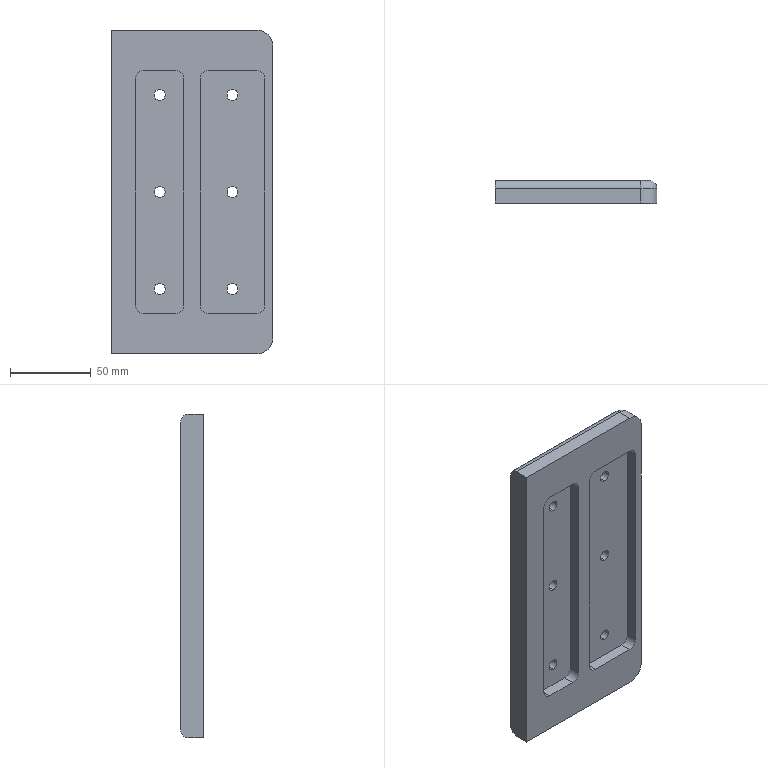Part | SolidWorks | features ICE 8, Fillet 3, HoleWzd 2, Chamfer 1, Extrusion 1, LPattern 1 | 1 solid | 43 faces | box 100 x 14 x 200 mm | volume 202593 mm3 | cylinder 25 | plane 16 | torus 2 | commonest cylinder face diameters 6.8 x12 10 x11 20 x2
STEP:
#1=CARTESIAN_POINT('',(-20.,14.,-63.4));
#2=VERTEX_POINT('',#1);
#3=CARTESIAN_POINT('',(-20.,14.,-56.6));
#4=VERTEX_POINT('',#3);
#5=CARTESIAN_POINT('',(-20.,14.,-60.));
#6=DIRECTION('',(0.,1.,0.));
#7=DIRECTION('',(0.,0.,1.));
#8=AXIS2_PLACEMENT_3D('',#5,#6,#7);
#9=CIRCLE('',#8,3.4);
#10=EDGE_CURVE('',#2,#4,#9,.T.);
#11=ORIENTED_EDGE('',*,*,#10,.T.);
#12=CARTESIAN_POINT('',(-20.,7.,-56.6));
#13=VERTEX_POINT('',#12);
#14=CARTESIAN_POINT('',(-20.,7.,-56.6));
#15=DIRECTION('',(0.,-1.,0.));
#16=VECTOR('',#15,1000.);
#17=LINE('',#14,#16);
#18=EDGE_CURVE('',#4,#13,#17,.T.);
#19=ORIENTED_EDGE('',*,*,#18,.T.);
#20=CARTESIAN_POINT('',(-20.,7.,-63.4));
#21=VERTEX_POINT('',#20);
#22=CARTESIAN_POINT('',(-20.,7.,-60.));
#23=DIRECTION('',(0.,-1.,0.));
#24=DIRECTION('',(0.,0.,-1.));
#25=AXIS2_PLACEMENT_3D('',#22,#23,#24);
#26=CIRCLE('',#25,3.4);
#27=EDGE_CURVE('',#13,#21,#26,.T.);
#28=ORIENTED_EDGE('',*,*,#27,.T.);
#29=CARTESIAN_POINT('',(-20.,7.,-63.4));
#30=DIRECTION('',(0.,-1.,0.));
#31=VECTOR('',#30,1000.);
#32=LINE('',#29,#31);
#33=EDGE_CURVE('',#2,#21,#32,.T.);
#34=ORIENTED_EDGE('',*,*,#33,.F.);
#35=EDGE_LOOP('',(#11,#19,#28,#34));
#36=FACE_OUTER_BOUND('',#35,.T.);
#37=CARTESIAN_POINT('',(-20.,7.,-60.));
#38=DIRECTION('',(0.,-1.,0.));
#39=DIRECTION('',(0.,0.,-1.));
#40=AXIS2_PLACEMENT_3D('',#37,#38,#39);
#41=CYLINDRICAL_SURFACE('',#40,3.4);
#42=ADVANCED_FACE('',(#36),#41,.F.);
#43=CARTESIAN_POINT('',(-20.,14.,-3.4));
#44=VERTEX_POINT('',#43);
#45=CARTESIAN_POINT('',(-20.,14.,3.4));
#46=VERTEX_POINT('',#45);
#47=CARTESIAN_POINT('',(-20.,14.,0.));
#48=DIRECTION('',(0.,1.,0.));
#49=DIRECTION('',(0.,0.,1.));
#50=AXIS2_PLACEMENT_3D('',#47,#48,#49);
#51=CIRCLE('',#50,3.4);
#52=EDGE_CURVE('',#44,#46,#51,.T.);
#53=ORIENTED_EDGE('',*,*,#52,.T.);
#54=CARTESIAN_POINT('',(-20.,7.,3.4));
#55=VERTEX_POINT('',#54);
#56=CARTESIAN_POINT('',(-20.,7.,3.4));
#57=DIRECTION('',(0.,-1.,0.));
#58=VECTOR('',#57,1000.);
#59=LINE('',#56,#58);
#60=EDGE_CURVE('',#46,#55,#59,.T.);
#61=ORIENTED_EDGE('',*,*,#60,.T.);
#62=CARTESIAN_POINT('',(-20.,7.,-3.4));
#63=VERTEX_POINT('',#62);
#64=CARTESIAN_POINT('',(-20.,7.,0.));
#65=DIRECTION('',(0.,-1.,0.));
#66=DIRECTION('',(0.,0.,-1.));
#67=AXIS2_PLACEMENT_3D('',#64,#65,#66);
#68=CIRCLE('',#67,3.4);
#69=EDGE_CURVE('',#55,#63,#68,.T.);
#70=ORIENTED_EDGE('',*,*,#69,.T.);
#71=CARTESIAN_POINT('',(-20.,7.,-3.4));
#72=DIRECTION('',(0.,-1.,0.));
#73=VECTOR('',#72,1000.);
#74=LINE('',#71,#73);
#75=EDGE_CURVE('',#44,#63,#74,.T.);
#76=ORIENTED_EDGE('',*,*,#75,.F.);
#77=EDGE_LOOP('',(#53,#61,#70,#76));
#78=FACE_OUTER_BOUND('',#77,.T.);
#79=CARTESIAN_POINT('',(-20.,7.,0.));
#80=DIRECTION('',(0.,-1.,0.));
#81=DIRECTION('',(0.,0.,-1.));
#82=AXIS2_PLACEMENT_3D('',#79,#80,#81);
#83=CYLINDRICAL_SURFACE('',#82,3.4);
#84=ADVANCED_FACE('',(#78),#83,.F.);
#85=CARTESIAN_POINT('',(-20.,14.,56.6));
#86=VERTEX_POINT('',#85);
#87=CARTESIAN_POINT('',(-20.,14.,63.4));
#88=VERTEX_POINT('',#87);
#89=CARTESIAN_POINT('',(-20.,14.,60.));
#90=DIRECTION('',(0.,1.,0.));
#91=DIRECTION('',(0.,0.,1.));
#92=AXIS2_PLACEMENT_3D('',#89,#90,#91);
#93=CIRCLE('',#92,3.4);
#94=EDGE_CURVE('',#86,#88,#93,.T.);
#95=ORIENTED_EDGE('',*,*,#94,.T.);
#96=CARTESIAN_POINT('',(-20.,7.,63.4));
#97=VERTEX_POINT('',#96);
#98=CARTESIAN_POINT('',(-20.,7.,63.4));
#99=DIRECTION('',(0.,-1.,0.));
#100=VECTOR('',#99,1000.);
#101=LINE('',#98,#100);
#102=EDGE_CURVE('',#88,#97,#101,.T.);
#103=ORIENTED_EDGE('',*,*,#102,.T.);
#104=CARTESIAN_POINT('',(-20.,7.,56.6));
#105=VERTEX_POINT('',#104);
#106=CARTESIAN_POINT('',(-20.,7.,60.));
#107=DIRECTION('',(0.,-1.,0.));
#108=DIRECTION('',(0.,0.,-1.));
#109=AXIS2_PLACEMENT_3D('',#106,#107,#108);
#110=CIRCLE('',#109,3.4);
#111=EDGE_CURVE('',#97,#105,#110,.T.);
#112=ORIENTED_EDGE('',*,*,#111,.T.);
#113=CARTESIAN_POINT('',(-20.,7.,56.6));
#114=DIRECTION('',(0.,-1.,0.));
#115=VECTOR('',#114,1000.);
#116=LINE('',#113,#115);
#117=EDGE_CURVE('',#86,#105,#116,.T.);
#118=ORIENTED_EDGE('',*,*,#117,.F.);
#119=EDGE_LOOP('',(#95,#103,#112,#118));
#120=FACE_OUTER_BOUND('',#119,.T.);
#121=CARTESIAN_POINT('',(-20.,7.,60.));
#122=DIRECTION('',(0.,-1.,0.));
#123=DIRECTION('',(0.,0.,-1.));
#124=AXIS2_PLACEMENT_3D('',#121,#122,#123);
#125=CYLINDRICAL_SURFACE('',#124,3.4);
#126=ADVANCED_FACE('',(#120),#125,.F.);
#127=CARTESIAN_POINT('',(25.,14.,-63.4));
#128=VERTEX_POINT('',#127);
#129=CARTESIAN_POINT('',(25.,14.,-56.6));
#130=VERTEX_POINT('',#129);
#131=CARTESIAN_POINT('',(25.,14.,-60.));
#132=DIRECTION('',(0.,1.,0.));
#133=DIRECTION('',(0.,0.,1.));
#134=AXIS2_PLACEMENT_3D('',#131,#132,#133);
#135=CIRCLE('',#134,3.4);
#136=EDGE_CURVE('',#128,#130,#135,.T.);
#137=ORIENTED_EDGE('',*,*,#136,.T.);
#138=CARTESIAN_POINT('',(25.,7.,-56.6));
#139=VERTEX_POINT('',#138);
#140=CARTESIAN_POINT('',(25.,7.,-56.6));
#141=DIRECTION('',(0.,-1.,0.));
#142=VECTOR('',#141,1000.);
#143=LINE('',#140,#142);
#144=EDGE_CURVE('',#130,#139,#143,.T.);
#145=ORIENTED_EDGE('',*,*,#144,.T.);
#146=CARTESIAN_POINT('',(25.,7.,-63.4));
#147=VERTEX_POINT('',#146);
#148=CARTESIAN_POINT('',(25.,7.,-60.));
#149=DIRECTION('',(0.,-1.,0.));
#150=DIRECTION('',(0.,0.,-1.));
#151=AXIS2_PLACEMENT_3D('',#148,#149,#150);
#152=CIRCLE('',#151,3.4);
#153=EDGE_CURVE('',#139,#147,#152,.T.);
#154=ORIENTED_EDGE('',*,*,#153,.T.);
#155=CARTESIAN_POINT('',(25.,7.,-63.4));
#156=DIRECTION('',(0.,-1.,0.));
#157=VECTOR('',#156,1000.);
#158=LINE('',#155,#157);
#159=EDGE_CURVE('',#128,#147,#158,.T.);
#160=ORIENTED_EDGE('',*,*,#159,.F.);
#161=EDGE_LOOP('',(#137,#145,#154,#160));
#162=FACE_OUTER_BOUND('',#161,.T.);
#163=CARTESIAN_POINT('',(25.,7.,-60.));
#164=DIRECTION('',(0.,-1.,0.));
#165=DIRECTION('',(0.,0.,-1.));
#166=AXIS2_PLACEMENT_3D('',#163,#164,#165);
#167=CYLINDRICAL_SURFACE('',#166,3.4);
#168=ADVANCED_FACE('',(#162),#167,.F.);
#169=CARTESIAN_POINT('',(25.,14.,-3.4));
#170=VERTEX_POINT('',#169);
#171=CARTESIAN_POINT('',(25.,14.,3.4));
#172=VERTEX_POINT('',#171);
#173=CARTESIAN_POINT('',(25.,14.,0.));
#174=DIRECTION('',(0.,1.,0.));
#175=DIRECTION('',(0.,0.,1.));
#176=AXIS2_PLACEMENT_3D('',#173,#174,#175);
#177=CIRCLE('',#176,3.4);
#178=EDGE_CURVE('',#170,#172,#177,.T.);
#179=ORIENTED_EDGE('',*,*,#178,.T.);
#180=CARTESIAN_POINT('',(25.,7.,3.4));
#181=VERTEX_POINT('',#180);
#182=CARTESIAN_POINT('',(25.,7.,3.4));
#183=DIRECTION('',(0.,-1.,0.));
#184=VECTOR('',#183,1000.);
#185=LINE('',#182,#184);
#186=EDGE_CURVE('',#172,#181,#185,.T.);
#187=ORIENTED_EDGE('',*,*,#186,.T.);
#188=CARTESIAN_POINT('',(25.,7.,-3.4));
#189=VERTEX_POINT('',#188);
#190=CARTESIAN_POINT('',(25.,7.,0.));
#191=DIRECTION('',(0.,-1.,0.));
#192=DIRECTION('',(0.,0.,-1.));
#193=AXIS2_PLACEMENT_3D('',#190,#191,#192);
#194=CIRCLE('',#193,3.4);
#195=EDGE_CURVE('',#181,#189,#194,.T.);
#196=ORIENTED_EDGE('',*,*,#195,.T.);
#197=CARTESIAN_POINT('',(25.,7.,-3.4));
#198=DIRECTION('',(0.,-1.,0.));
#199=VECTOR('',#198,1000.);
#200=LINE('',#197,#199);
#201=EDGE_CURVE('',#170,#189,#200,.T.);
#202=ORIENTED_EDGE('',*,*,#201,.F.);
#203=EDGE_LOOP('',(#179,#187,#196,#202));
#204=FACE_OUTER_BOUND('',#203,.T.);
#205=CARTESIAN_POINT('',(25.,7.,0.));
#206=DIRECTION('',(0.,-1.,0.));
#207=DIRECTION('',(0.,0.,-1.));
#208=AXIS2_PLACEMENT_3D('',#205,#206,#207);
#209=CYLINDRICAL_SURFACE('',#208,3.4);
#210=ADVANCED_FACE('',(#204),#209,.F.);
#211=CARTESIAN_POINT('',(25.,14.,56.6));
#212=VERTEX_POINT('',#211);
#213=CARTESIAN_POINT('',(25.,14.,63.4));
#214=VERTEX_POINT('',#213);
#215=CARTESIAN_POINT('',(25.,14.,60.));
#216=DIRECTION('',(0.,1.,0.));
#217=DIRECTION('',(0.,0.,1.));
#218=AXIS2_PLACEMENT_3D('',#215,#216,#217);
#219=CIRCLE('',#218,3.4);
#220=EDGE_CURVE('',#212,#214,#219,.T.);
#221=ORIENTED_EDGE('',*,*,#220,.T.);
#222=CARTESIAN_POINT('',(25.,7.,63.4));
#223=VERTEX_POINT('',#222);
#224=CARTESIAN_POINT('',(25.,7.,63.4));
#225=DIRECTION('',(0.,-1.,0.));
#226=VECTOR('',#225,1000.);
#227=LINE('',#224,#226);
#228=EDGE_CURVE('',#214,#223,#227,.T.);
#229=ORIENTED_EDGE('',*,*,#228,.T.);
#230=CARTESIAN_POINT('',(25.,7.,56.6));
#231=VERTEX_POINT('',#230);
#232=CARTESIAN_POINT('',(25.,7.,60.));
#233=DIRECTION('',(0.,-1.,0.));
#234=DIRECTION('',(0.,0.,-1.));
#235=AXIS2_PLACEMENT_3D('',#232,#233,#234);
#236=CIRCLE('',#235,3.4);
#237=EDGE_CURVE('',#223,#231,#236,.T.);
#238=ORIENTED_EDGE('',*,*,#237,.T.);
#239=CARTESIAN_POINT('',(25.,7.,56.6));
#240=DIRECTION('',(0.,-1.,0.));
#241=VECTOR('',#240,1000.);
#242=LINE('',#239,#241);
#243=EDGE_CURVE('',#212,#231,#242,.T.);
#244=ORIENTED_EDGE('',*,*,#243,.F.);
#245=EDGE_LOOP('',(#221,#229,#238,#244));
#246=FACE_OUTER_BOUND('',#245,.T.);
#247=CARTESIAN_POINT('',(25.,7.,60.));
#248=DIRECTION('',(0.,-1.,0.));
#249=DIRECTION('',(0.,0.,-1.));
#250=AXIS2_PLACEMENT_3D('',#247,#248,#249);
#251=CYLINDRICAL_SURFACE('',#250,3.4);
#252=ADVANCED_FACE('',(#246),#251,.F.);
#253=CARTESIAN_POINT('',(-30.,0.,-75.));
#254=VERTEX_POINT('',#253);
#255=CARTESIAN_POINT('',(-10.,0.,-75.));
#256=VERTEX_POINT('',#255);
#257=CARTESIAN_POINT('',(-45.,0.,-75.));
#258=DIRECTION('',(1.,0.,0.));
#259=VECTOR('',#258,1000.);
#260=LINE('',#257,#259);
#261=EDGE_CURVE('',#254,#256,#260,.T.);
#262=ORIENTED_EDGE('',*,*,#261,.F.);
#263=CARTESIAN_POINT('',(-35.,0.,-70.));
#264=VERTEX_POINT('',#263);
#265=CARTESIAN_POINT('',(-30.,0.,-70.));
#266=DIRECTION('',(0.,1.,0.));
#267=DIRECTION('',(0.,0.,1.));
#268=AXIS2_PLACEMENT_3D('',#265,#266,#267);
#269=CIRCLE('',#268,5.);
#270=EDGE_CURVE('',#254,#264,#269,.T.);
#271=ORIENTED_EDGE('',*,*,#270,.T.);
#272=CARTESIAN_POINT('',(-35.,0.,70.));
#273=VERTEX_POINT('',#272);
#274=CARTESIAN_POINT('',(-35.,0.,75.));
#275=DIRECTION('',(0.,0.,1.));
#276=VECTOR('',#275,1000.);
#277=LINE('',#274,#276);
#278=EDGE_CURVE('',#264,#273,#277,.T.);
#279=ORIENTED_EDGE('',*,*,#278,.T.);
#280=CARTESIAN_POINT('',(-30.,0.,75.));
#281=VERTEX_POINT('',#280);
#282=CARTESIAN_POINT('',(-30.,0.,70.));
#283=DIRECTION('',(0.,1.,0.));
#284=DIRECTION('',(0.,0.,1.));
#285=AXIS2_PLACEMENT_3D('',#282,#283,#284);
#286=CIRCLE('',#285,5.);
#287=EDGE_CURVE('',#273,#281,#286,.T.);
#288=ORIENTED_EDGE('',*,*,#287,.T.);
#289=CARTESIAN_POINT('',(-10.,0.,75.));
#290=VERTEX_POINT('',#289);
#291=CARTESIAN_POINT('',(-45.,0.,75.));
#292=DIRECTION('',(-1.,0.,0.));
#293=VECTOR('',#292,1000.);
#294=LINE('',#291,#293);
#295=EDGE_CURVE('',#290,#281,#294,.T.);
#296=ORIENTED_EDGE('',*,*,#295,.F.);
#297=CARTESIAN_POINT('',(-5.,0.,70.));
#298=VERTEX_POINT('',#297);
#299=CARTESIAN_POINT('',(-10.,0.,70.));
#300=DIRECTION('',(0.,1.,0.));
#301=DIRECTION('',(0.,0.,1.));
#302=AXIS2_PLACEMENT_3D('',#299,#300,#301);
#303=CIRCLE('',#302,5.);
#304=EDGE_CURVE('',#290,#298,#303,.T.);
#305=ORIENTED_EDGE('',*,*,#304,.T.);
#306=CARTESIAN_POINT('',(-5.,0.,-70.));
#307=VERTEX_POINT('',#306);
#308=CARTESIAN_POINT('',(-5.,0.,75.));
#309=DIRECTION('',(0.,0.,1.));
#310=VECTOR('',#309,1000.);
#311=LINE('',#308,#310);
#312=EDGE_CURVE('',#307,#298,#311,.T.);
#313=ORIENTED_EDGE('',*,*,#312,.F.);
#314=CARTESIAN_POINT('',(-10.,0.,-70.));
#315=DIRECTION('',(0.,1.,0.));
#316=DIRECTION('',(0.,0.,1.));
#317=AXIS2_PLACEMENT_3D('',#314,#315,#316);
#318=CIRCLE('',#317,5.);
#319=EDGE_CURVE('',#307,#256,#318,.T.);
#320=ORIENTED_EDGE('',*,*,#319,.T.);
#321=EDGE_LOOP('',(#262,#271,#279,#288,#296,#305,#313,#320));
#322=FACE_BOUND('',#321,.T.);
#323=CARTESIAN_POINT('',(40.,0.,-100.));
#324=VERTEX_POINT('',#323);
#325=CARTESIAN_POINT('',(-50.,0.,-100.));
#326=VERTEX_POINT('',#325);
#327=CARTESIAN_POINT('',(-50.,0.,-100.));
#328=DIRECTION('',(-1.,0.,0.));
#329=VECTOR('',#328,1000.);
#330=LINE('',#327,#329);
#331=EDGE_CURVE('',#324,#326,#330,.T.);
#332=ORIENTED_EDGE('',*,*,#331,.F.);
#333=CARTESIAN_POINT('',(50.,0.,-90.));
#334=VERTEX_POINT('',#333);
#335=CARTESIAN_POINT('',(40.,0.,-90.));
#336=DIRECTION('',(0.,-1.,0.));
#337=DIRECTION('',(0.,0.,1.));
#338=AXIS2_PLACEMENT_3D('',#335,#336,#337);
#339=CIRCLE('',#338,10.);
#340=EDGE_CURVE('',#324,#334,#339,.T.);
#341=ORIENTED_EDGE('',*,*,#340,.T.);
#342=CARTESIAN_POINT('',(50.,0.,90.));
#343=VERTEX_POINT('',#342);
#344=CARTESIAN_POINT('',(50.,0.,-100.));
#345=DIRECTION('',(0.,0.,-1.));
#346=VECTOR('',#345,1000.);
#347=LINE('',#344,#346);
#348=EDGE_CURVE('',#343,#334,#347,.T.);
#349=ORIENTED_EDGE('',*,*,#348,.F.);
#350=CARTESIAN_POINT('',(40.,0.,100.));
#351=VERTEX_POINT('',#350);
#352=CARTESIAN_POINT('',(40.,0.,90.));
#353=DIRECTION('',(0.,-1.,0.));
#354=DIRECTION('',(0.,0.,1.));
#355=AXIS2_PLACEMENT_3D('',#352,#353,#354);
#356=CIRCLE('',#355,10.);
#357=EDGE_CURVE('',#343,#351,#356,.T.);
#358=ORIENTED_EDGE('',*,*,#357,.T.);
#359=CARTESIAN_POINT('',(-50.,0.,100.));
#360=VERTEX_POINT('',#359);
#361=CARTESIAN_POINT('',(-50.,0.,100.));
#362=DIRECTION('',(1.,0.,0.));
#363=VECTOR('',#362,1000.);
#364=LINE('',#361,#363);
#365=EDGE_CURVE('',#360,#351,#364,.T.);
#366=ORIENTED_EDGE('',*,*,#365,.F.);
#367=CARTESIAN_POINT('',(-50.,0.,-100.));
#368=DIRECTION('',(0.,0.,1.));
#369=VECTOR('',#368,1000.);
#370=LINE('',#367,#369);
#371=EDGE_CURVE('',#326,#360,#370,.T.);
#372=ORIENTED_EDGE('',*,*,#371,.F.);
#373=EDGE_LOOP('',(#332,#341,#349,#358,#366,#372));
#374=FACE_OUTER_BOUND('',#373,.T.);
#375=CARTESIAN_POINT('',(40.,0.,75.));
#376=VERTEX_POINT('',#375);
#377=CARTESIAN_POINT('',(10.,0.,75.));
#378=VERTEX_POINT('',#377);
#379=CARTESIAN_POINT('',(45.,0.,75.));
#380=DIRECTION('',(-1.,0.,0.));
#381=VECTOR('',#380,1000.);
#382=LINE('',#379,#381);
#383=EDGE_CURVE('',#376,#378,#382,.T.);
#384=ORIENTED_EDGE('',*,*,#383,.F.);
#385=CARTESIAN_POINT('',(45.,0.,70.));
#386=VERTEX_POINT('',#385);
#387=CARTESIAN_POINT('',(40.,0.,70.));
#388=DIRECTION('',(0.,1.,0.));
#389=DIRECTION('',(0.,0.,1.));
#390=AXIS2_PLACEMENT_3D('',#387,#388,#389);
#391=CIRCLE('',#390,5.);
#392=EDGE_CURVE('',#376,#386,#391,.T.);
#393=ORIENTED_EDGE('',*,*,#392,.T.);
#394=CARTESIAN_POINT('',(45.,0.,-70.));
#395=VERTEX_POINT('',#394);
#396=CARTESIAN_POINT('',(45.,0.,75.));
#397=DIRECTION('',(0.,0.,1.));
#398=VECTOR('',#397,1000.);
#399=LINE('',#396,#398);
#400=EDGE_CURVE('',#395,#386,#399,.T.);
#401=ORIENTED_EDGE('',*,*,#400,.F.);
#402=CARTESIAN_POINT('',(40.,0.,-75.));
#403=VERTEX_POINT('',#402);
#404=CARTESIAN_POINT('',(40.,0.,-70.));
#405=DIRECTION('',(0.,1.,0.));
#406=DIRECTION('',(0.,0.,1.));
#407=AXIS2_PLACEMENT_3D('',#404,#405,#406);
#408=CIRCLE('',#407,5.);
#409=EDGE_CURVE('',#395,#403,#408,.T.);
#410=ORIENTED_EDGE('',*,*,#409,.T.);
#411=CARTESIAN_POINT('',(10.,0.,-75.));
#412=VERTEX_POINT('',#411);
#413=CARTESIAN_POINT('',(45.,0.,-75.));
#414=DIRECTION('',(1.,0.,0.));
#415=VECTOR('',#414,1000.);
#416=LINE('',#413,#415);
#417=EDGE_CURVE('',#412,#403,#416,.T.);
#418=ORIENTED_EDGE('',*,*,#417,.F.);
#419=CARTESIAN_POINT('',(5.,0.,-70.));
#420=VERTEX_POINT('',#419);
#421=CARTESIAN_POINT('',(10.,0.,-70.));
#422=DIRECTION('',(0.,1.,0.));
#423=DIRECTION('',(0.,0.,1.));
#424=AXIS2_PLACEMENT_3D('',#421,#422,#423);
#425=CIRCLE('',#424,5.);
#426=EDGE_CURVE('',#412,#420,#425,.T.);
#427=ORIENTED_EDGE('',*,*,#426,.T.);
#428=CARTESIAN_POINT('',(5.,0.,70.));
#429=VERTEX_POINT('',#428);
#430=CARTESIAN_POINT('',(5.,0.,75.));
#431=DIRECTION('',(0.,0.,-1.));
#432=VECTOR('',#431,1000.);
#433=LINE('',#430,#432);
#434=EDGE_CURVE('',#429,#420,#433,.T.);
#435=ORIENTED_EDGE('',*,*,#434,.F.);
#436=CARTESIAN_POINT('',(10.,0.,70.));
#437=DIRECTION('',(0.,1.,0.));
#438=DIRECTION('',(0.,0.,1.));
#439=AXIS2_PLACEMENT_3D('',#436,#437,#438);
#440=CIRCLE('',#439,5.);
#441=EDGE_CURVE('',#429,#378,#440,.T.);
#442=ORIENTED_EDGE('',*,*,#441,.T.);
#443=EDGE_LOOP('',(#384,#393,#401,#410,#418,#427,#435,#442));
#444=FACE_BOUND('',#443,.T.);
#445=CARTESIAN_POINT('',(0.,0.,0.));
#446=DIRECTION('',(0.,1.,0.));
#447=DIRECTION('',(0.,0.,1.));
#448=AXIS2_PLACEMENT_3D('',#445,#446,#447);
#449=PLANE('',#448);
#450=ADVANCED_FACE('',(#322,#374,#444),#449,.F.);
#451=CARTESIAN_POINT('',(50.,9.,-90.));
#452=VERTEX_POINT('',#451);
#453=CARTESIAN_POINT('',(50.,14.,-90.));
#454=DIRECTION('',(0.,1.,0.));
#455=VECTOR('',#454,1000.);
#456=LINE('',#453,#455);
#457=EDGE_CURVE('',#334,#452,#456,.T.);
#458=ORIENTED_EDGE('',*,*,#457,.T.);
#459=CARTESIAN_POINT('',(50.,9.,90.));
#460=VERTEX_POINT('',#459);
#461=CARTESIAN_POINT('',(50.,9.,90.));
#462=DIRECTION('',(0.,0.,1.));
#463=VECTOR('',#462,1000.);
#464=LINE('',#461,#463);
#465=EDGE_CURVE('',#452,#460,#464,.T.);
#466=ORIENTED_EDGE('',*,*,#465,.T.);
#467=CARTESIAN_POINT('',(50.,14.,90.));
#468=DIRECTION('',(0.,-1.,0.));
#469=VECTOR('',#468,1000.);
#470=LINE('',#467,#469);
#471=EDGE_CURVE('',#460,#343,#470,.T.);
#472=ORIENTED_EDGE('',*,*,#471,.T.);
#473=ORIENTED_EDGE('',*,*,#348,.T.);
#474=EDGE_LOOP('',(#458,#466,#472,#473));
#475=FACE_OUTER_BOUND('',#474,.T.);
#476=CARTESIAN_POINT('',(50.,14.,-100.));
#477=DIRECTION('',(-1.,0.,0.));
#478=DIRECTION('',(0.,0.,1.));
#479=AXIS2_PLACEMENT_3D('',#476,#477,#478);
#480=PLANE('',#479);
#481=ADVANCED_FACE('',(#475),#480,.F.);
#482=CARTESIAN_POINT('',(-50.,9.,-100.));
#483=VERTEX_POINT('',#482);
#484=CARTESIAN_POINT('',(-50.,14.,-100.));
#485=DIRECTION('',(0.,-1.,0.));
#486=VECTOR('',#485,1000.);
#487=LINE('',#484,#486);
#488=EDGE_CURVE('',#483,#326,#487,.T.);
#489=ORIENTED_EDGE('',*,*,#488,.F.);
#490=CARTESIAN_POINT('',(40.,9.,-100.));
#491=VERTEX_POINT('',#490);
#492=CARTESIAN_POINT('',(40.,9.,-100.));
#493=DIRECTION('',(1.,0.,0.));
#494=VECTOR('',#493,1000.);
#495=LINE('',#492,#494);
#496=EDGE_CURVE('',#483,#491,#495,.T.);
#497=ORIENTED_EDGE('',*,*,#496,.T.);
#498=CARTESIAN_POINT('',(40.,14.,-100.));
#499=DIRECTION('',(0.,-1.,0.));
#500=VECTOR('',#499,1000.);
#501=LINE('',#498,#500);
#502=EDGE_CURVE('',#491,#324,#501,.T.);
#503=ORIENTED_EDGE('',*,*,#502,.T.);
#504=ORIENTED_EDGE('',*,*,#331,.T.);
#505=EDGE_LOOP('',(#489,#497,#503,#504));
#506=FACE_OUTER_BOUND('',#505,.T.);
#507=CARTESIAN_POINT('',(-50.,14.,-100.));
#508=DIRECTION('',(0.,0.,1.));
#509=DIRECTION('',(1.,0.,0.));
#510=AXIS2_PLACEMENT_3D('',#507,#508,#509);
#511=PLANE('',#510);
#512=ADVANCED_FACE('',(#506),#511,.F.);
#513=CARTESIAN_POINT('',(-50.,9.,100.));
#514=VERTEX_POINT('',#513);
#515=CARTESIAN_POINT('',(-50.,14.,100.));
#516=DIRECTION('',(0.,-1.,0.));
#517=VECTOR('',#516,1000.);
#518=LINE('',#515,#517);
#519=EDGE_CURVE('',#514,#360,#518,.T.);
#520=ORIENTED_EDGE('',*,*,#519,.F.);
#521=CARTESIAN_POINT('',(-50.,14.,95.));
#522=VERTEX_POINT('',#521);
#523=CARTESIAN_POINT('',(-50.,9.,95.));
#524=DIRECTION('',(-1.,0.,0.));
#525=DIRECTION('',(0.,0.,-1.));
#526=AXIS2_PLACEMENT_3D('',#523,#524,#525);
#527=CIRCLE('',#526,5.);
#528=EDGE_CURVE('',#514,#522,#527,.T.);
#529=ORIENTED_EDGE('',*,*,#528,.T.);
#530=CARTESIAN_POINT('',(-50.,14.,-95.));
#531=VERTEX_POINT('',#530);
#532=CARTESIAN_POINT('',(-50.,14.,-100.));
#533=DIRECTION('',(0.,0.,1.));
#534=VECTOR('',#533,1000.);
#535=LINE('',#532,#534);
#536=EDGE_CURVE('',#531,#522,#535,.T.);
#537=ORIENTED_EDGE('',*,*,#536,.F.);
#538=CARTESIAN_POINT('',(-50.,9.,-95.));
#539=DIRECTION('',(-1.,0.,0.));
#540=DIRECTION('',(0.,0.,-1.));
#541=AXIS2_PLACEMENT_3D('',#538,#539,#540);
#542=CIRCLE('',#541,5.);
#543=EDGE_CURVE('',#531,#483,#542,.T.);
#544=ORIENTED_EDGE('',*,*,#543,.T.);
#545=ORIENTED_EDGE('',*,*,#488,.T.);
#546=ORIENTED_EDGE('',*,*,#371,.T.);
#547=EDGE_LOOP('',(#520,#529,#537,#544,#545,#546));
#548=FACE_OUTER_BOUND('',#547,.T.);
#549=CARTESIAN_POINT('',(-50.,14.,-100.));
#550=DIRECTION('',(1.,0.,0.));
#551=DIRECTION('',(0.,0.,-1.));
#552=AXIS2_PLACEMENT_3D('',#549,#550,#551);
#553=PLANE('',#552);
#554=ADVANCED_FACE('',(#548),#553,.F.);
#555=CARTESIAN_POINT('',(40.,9.,100.));
#556=VERTEX_POINT('',#555);
#557=CARTESIAN_POINT('',(40.,14.,100.));
#558=DIRECTION('',(0.,1.,0.));
#559=VECTOR('',#558,1000.);
#560=LINE('',#557,#559);
#561=EDGE_CURVE('',#351,#556,#560,.T.);
#562=ORIENTED_EDGE('',*,*,#561,.T.);
#563=CARTESIAN_POINT('',(-50.,9.,100.));
#564=DIRECTION('',(-1.,0.,0.));
#565=VECTOR('',#564,1000.);
#566=LINE('',#563,#565);
#567=EDGE_CURVE('',#556,#514,#566,.T.);
#568=ORIENTED_EDGE('',*,*,#567,.T.);
#569=ORIENTED_EDGE('',*,*,#519,.T.);
#570=ORIENTED_EDGE('',*,*,#365,.T.);
#571=EDGE_LOOP('',(#562,#568,#569,#570));
#572=FACE_OUTER_BOUND('',#571,.T.);
#573=CARTESIAN_POINT('',(-50.,14.,100.));
#574=DIRECTION('',(0.,0.,-1.));
#575=DIRECTION('',(-1.,0.,0.));
#576=AXIS2_PLACEMENT_3D('',#573,#574,#575);
#577=PLANE('',#576);
#578=ADVANCED_FACE('',(#572),#577,.F.);
#579=ORIENTED_EDGE('',*,*,#10,.F.);
#580=CARTESIAN_POINT('',(-20.,14.,-60.));
#581=DIRECTION('',(0.,1.,0.));
#582=DIRECTION('',(0.,0.,1.));
#583=AXIS2_PLACEMENT_3D('',#580,#581,#582);
#584=CIRCLE('',#583,3.4);
#585=EDGE_CURVE('',#4,#2,#584,.T.);
#586=ORIENTED_EDGE('',*,*,#585,.F.);
#587=EDGE_LOOP('',(#579,#586));
#588=FACE_BOUND('',#587,.T.);
#589=ORIENTED_EDGE('',*,*,#52,.F.);
#590=CARTESIAN_POINT('',(-20.,14.,0.));
#591=DIRECTION('',(0.,1.,0.));
#592=DIRECTION('',(0.,0.,1.));
#593=AXIS2_PLACEMENT_3D('',#590,#591,#592);
#594=CIRCLE('',#593,3.4);
#595=EDGE_CURVE('',#46,#44,#594,.T.);
#596=ORIENTED_EDGE('',*,*,#595,.F.);
#597=EDGE_LOOP('',(#589,#596));
#598=FACE_BOUND('',#597,.T.);
#599=ORIENTED_EDGE('',*,*,#94,.F.);
#600=CARTESIAN_POINT('',(-20.,14.,60.));
#601=DIRECTION('',(0.,1.,0.));
#602=DIRECTION('',(0.,0.,1.));
#603=AXIS2_PLACEMENT_3D('',#600,#601,#602);
#604=CIRCLE('',#603,3.4);
#605=EDGE_CURVE('',#88,#86,#604,.T.);
#606=ORIENTED_EDGE('',*,*,#605,.F.);
#607=EDGE_LOOP('',(#599,#606));
#608=FACE_BOUND('',#607,.T.);
#609=ORIENTED_EDGE('',*,*,#136,.F.);
#610=CARTESIAN_POINT('',(25.,14.,-60.));
#611=DIRECTION('',(0.,1.,0.));
#612=DIRECTION('',(0.,0.,1.));
#613=AXIS2_PLACEMENT_3D('',#610,#611,#612);
#614=CIRCLE('',#613,3.4);
#615=EDGE_CURVE('',#130,#128,#614,.T.);
#616=ORIENTED_EDGE('',*,*,#615,.F.);
#617=EDGE_LOOP('',(#609,#616));
#618=FACE_BOUND('',#617,.T.);
#619=ORIENTED_EDGE('',*,*,#178,.F.);
#620=CARTESIAN_POINT('',(25.,14.,0.));
#621=DIRECTION('',(0.,1.,0.));
#622=DIRECTION('',(0.,0.,1.));
#623=AXIS2_PLACEMENT_3D('',#620,#621,#622);
#624=CIRCLE('',#623,3.4);
#625=EDGE_CURVE('',#172,#170,#624,.T.);
#626=ORIENTED_EDGE('',*,*,#625,.F.);
#627=EDGE_LOOP('',(#619,#626));
#628=FACE_BOUND('',#627,.T.);
#629=ORIENTED_EDGE('',*,*,#220,.F.);
#630=CARTESIAN_POINT('',(25.,14.,60.));
#631=DIRECTION('',(0.,1.,0.));
#632=DIRECTION('',(0.,0.,1.));
#633=AXIS2_PLACEMENT_3D('',#630,#631,#632);
#634=CIRCLE('',#633,3.4);
#635=EDGE_CURVE('',#214,#212,#634,.T.);
#636=ORIENTED_EDGE('',*,*,#635,.F.);
#637=EDGE_LOOP('',(#629,#636));
#638=FACE_BOUND('',#637,.T.);
#639=ORIENTED_EDGE('',*,*,#536,.T.);
#640=CARTESIAN_POINT('',(40.,14.,95.));
#641=VERTEX_POINT('',#640);
#642=CARTESIAN_POINT('',(40.,14.,95.));
#643=DIRECTION('',(1.,0.,0.));
#644=VECTOR('',#643,1000.);
#645=LINE('',#642,#644);
#646=EDGE_CURVE('',#522,#641,#645,.T.);
#647=ORIENTED_EDGE('',*,*,#646,.T.);
#648=CARTESIAN_POINT('',(45.,14.,90.));
#649=VERTEX_POINT('',#648);
#650=CARTESIAN_POINT('',(40.,14.,90.));
#651=DIRECTION('',(0.,1.,0.));
#652=DIRECTION('',(0.,0.,1.));
#653=AXIS2_PLACEMENT_3D('',#650,#651,#652);
#654=CIRCLE('',#653,5.);
#655=EDGE_CURVE('',#641,#649,#654,.T.);
#656=ORIENTED_EDGE('',*,*,#655,.T.);
#657=CARTESIAN_POINT('',(45.,14.,-90.));
#658=VERTEX_POINT('',#657);
#659=CARTESIAN_POINT('',(45.,14.,-90.));
#660=DIRECTION('',(0.,0.,-1.));
#661=VECTOR('',#660,1000.);
#662=LINE('',#659,#661);
#663=EDGE_CURVE('',#649,#658,#662,.T.);
#664=ORIENTED_EDGE('',*,*,#663,.T.);
#665=CARTESIAN_POINT('',(40.,14.,-95.));
#666=VERTEX_POINT('',#665);
#667=CARTESIAN_POINT('',(40.,14.,-90.));
#668=DIRECTION('',(0.,1.,0.));
#669=DIRECTION('',(0.,0.,1.));
#670=AXIS2_PLACEMENT_3D('',#667,#668,#669);
#671=CIRCLE('',#670,5.);
#672=EDGE_CURVE('',#658,#666,#671,.T.);
#673=ORIENTED_EDGE('',*,*,#672,.T.);
#674=CARTESIAN_POINT('',(-50.,14.,-95.));
#675=DIRECTION('',(-1.,0.,0.));
#676=VECTOR('',#675,1000.);
#677=LINE('',#674,#676);
#678=EDGE_CURVE('',#666,#531,#677,.T.);
#679=ORIENTED_EDGE('',*,*,#678,.T.);
#680=EDGE_LOOP('',(#639,#647,#656,#664,#673,#679));
#681=FACE_OUTER_BOUND('',#680,.T.);
#682=CARTESIAN_POINT('',(0.,14.,0.));
#683=DIRECTION('',(0.,1.,0.));
#684=DIRECTION('',(0.,0.,1.));
#685=AXIS2_PLACEMENT_3D('',#682,#683,#684);
#686=PLANE('',#685);
#687=ADVANCED_FACE('',(#588,#598,#608,#618,#628,#638,#681),#686,.T.);
#688=ORIENTED_EDGE('',*,*,#502,.F.);
#689=CARTESIAN_POINT('',(40.,9.,-90.));
#690=DIRECTION('',(0.,-1.,0.));
#691=DIRECTION('',(0.,0.,1.));
#692=AXIS2_PLACEMENT_3D('',#689,#690,#691);
#693=CIRCLE('',#692,10.);
#694=EDGE_CURVE('',#491,#452,#693,.T.);
#695=ORIENTED_EDGE('',*,*,#694,.T.);
#696=ORIENTED_EDGE('',*,*,#457,.F.);
#697=ORIENTED_EDGE('',*,*,#340,.F.);
#698=EDGE_LOOP('',(#688,#695,#696,#697));
#699=FACE_OUTER_BOUND('',#698,.T.);
#700=CARTESIAN_POINT('',(40.,14.,-90.));
#701=DIRECTION('',(0.,-1.,0.));
#702=DIRECTION('',(0.,0.,-1.));
#703=AXIS2_PLACEMENT_3D('',#700,#701,#702);
#704=CYLINDRICAL_SURFACE('',#703,10.);
#705=ADVANCED_FACE('',(#699),#704,.T.);
#706=ORIENTED_EDGE('',*,*,#471,.F.);
#707=CARTESIAN_POINT('',(40.,9.,90.));
#708=DIRECTION('',(0.,-1.,0.));
#709=DIRECTION('',(0.,0.,1.));
#710=AXIS2_PLACEMENT_3D('',#707,#708,#709);
#711=CIRCLE('',#710,10.);
#712=EDGE_CURVE('',#460,#556,#711,.T.);
#713=ORIENTED_EDGE('',*,*,#712,.T.);
#714=ORIENTED_EDGE('',*,*,#561,.F.);
#715=ORIENTED_EDGE('',*,*,#357,.F.);
#716=EDGE_LOOP('',(#706,#713,#714,#715));
#717=FACE_OUTER_BOUND('',#716,.T.);
#718=CARTESIAN_POINT('',(40.,14.,90.));
#719=DIRECTION('',(0.,-1.,0.));
#720=DIRECTION('',(0.,0.,-1.));
#721=AXIS2_PLACEMENT_3D('',#718,#719,#720);
#722=CYLINDRICAL_SURFACE('',#721,10.);
#723=ADVANCED_FACE('',(#717),#722,.T.);
#724=ORIENTED_EDGE('',*,*,#543,.F.);
#725=ORIENTED_EDGE('',*,*,#678,.F.);
#726=CARTESIAN_POINT('',(40.,9.,-95.));
#727=DIRECTION('',(1.,0.,0.));
#728=DIRECTION('',(0.,0.,-1.));
#729=AXIS2_PLACEMENT_3D('',#726,#727,#728);
#730=CIRCLE('',#729,5.);
#731=EDGE_CURVE('',#491,#666,#730,.T.);
#732=ORIENTED_EDGE('',*,*,#731,.F.);
#733=ORIENTED_EDGE('',*,*,#496,.F.);
#734=EDGE_LOOP('',(#724,#725,#732,#733));
#735=FACE_OUTER_BOUND('',#734,.T.);
#736=CARTESIAN_POINT('',(0.,9.,-95.));
#737=DIRECTION('',(1.,0.,0.));
#738=DIRECTION('',(0.,0.,-1.));
#739=AXIS2_PLACEMENT_3D('',#736,#737,#738);
#740=CYLINDRICAL_SURFACE('',#739,5.);
#741=ADVANCED_FACE('',(#735),#740,.T.);
#742=ORIENTED_EDGE('',*,*,#731,.T.);
#743=ORIENTED_EDGE('',*,*,#672,.F.);
#744=CARTESIAN_POINT('',(45.,9.,-90.));
#745=DIRECTION('',(0.,0.,1.));
#746=DIRECTION('',(1.,0.,0.));
#747=AXIS2_PLACEMENT_3D('',#744,#745,#746);
#748=CIRCLE('',#747,5.);
#749=EDGE_CURVE('',#452,#658,#748,.T.);
#750=ORIENTED_EDGE('',*,*,#749,.F.);
#751=ORIENTED_EDGE('',*,*,#694,.F.);
#752=EDGE_LOOP('',(#742,#743,#750,#751));
#753=FACE_OUTER_BOUND('',#752,.T.);
#754=CARTESIAN_POINT('',(40.,9.,-90.));
#755=DIRECTION('',(0.,1.,0.));
#756=DIRECTION('',(0.,0.,1.));
#757=AXIS2_PLACEMENT_3D('',#754,#755,#756);
#758=TOROIDAL_SURFACE('',#757,5.,5.);
#759=ADVANCED_FACE('',(#753),#758,.T.);
#760=ORIENTED_EDGE('',*,*,#749,.T.);
#761=ORIENTED_EDGE('',*,*,#663,.F.);
#762=CARTESIAN_POINT('',(45.,9.,90.));
#763=DIRECTION('',(0.,0.,1.));
#764=DIRECTION('',(1.,0.,0.));
#765=AXIS2_PLACEMENT_3D('',#762,#763,#764);
#766=CIRCLE('',#765,5.);
#767=EDGE_CURVE('',#460,#649,#766,.T.);
#768=ORIENTED_EDGE('',*,*,#767,.F.);
#769=ORIENTED_EDGE('',*,*,#465,.F.);
#770=EDGE_LOOP('',(#760,#761,#768,#769));
#771=FACE_OUTER_BOUND('',#770,.T.);
#772=CARTESIAN_POINT('',(45.,9.,0.));
#773=DIRECTION('',(0.,0.,1.));
#774=DIRECTION('',(1.,0.,0.));
#775=AXIS2_PLACEMENT_3D('',#772,#773,#774);
#776=CYLINDRICAL_SURFACE('',#775,5.);
#777=ADVANCED_FACE('',(#771),#776,.T.);
#778=ORIENTED_EDGE('',*,*,#767,.T.);
#779=ORIENTED_EDGE('',*,*,#655,.F.);
#780=CARTESIAN_POINT('',(40.,9.,95.));
#781=DIRECTION('',(-1.,0.,0.));
#782=DIRECTION('',(0.,0.,1.));
#783=AXIS2_PLACEMENT_3D('',#780,#781,#782);
#784=CIRCLE('',#783,5.);
#785=EDGE_CURVE('',#556,#641,#784,.T.);
#786=ORIENTED_EDGE('',*,*,#785,.F.);
#787=ORIENTED_EDGE('',*,*,#712,.F.);
#788=EDGE_LOOP('',(#778,#779,#786,#787));
#789=FACE_OUTER_BOUND('',#788,.T.);
#790=CARTESIAN_POINT('',(40.,9.,90.));
#791=DIRECTION('',(0.,1.,0.));
#792=DIRECTION('',(0.,0.,1.));
#793=AXIS2_PLACEMENT_3D('',#790,#791,#792);
#794=TOROIDAL_SURFACE('',#793,5.,5.);
#795=ADVANCED_FACE('',(#789),#794,.T.);
#796=ORIENTED_EDGE('',*,*,#528,.F.);
#797=ORIENTED_EDGE('',*,*,#567,.F.);
#798=ORIENTED_EDGE('',*,*,#785,.T.);
#799=ORIENTED_EDGE('',*,*,#646,.F.);
#800=EDGE_LOOP('',(#796,#797,#798,#799));
#801=FACE_OUTER_BOUND('',#800,.T.);
#802=CARTESIAN_POINT('',(0.,9.,95.));
#803=DIRECTION('',(-1.,0.,0.));
#804=DIRECTION('',(0.,0.,1.));
#805=AXIS2_PLACEMENT_3D('',#802,#803,#804);
#806=CYLINDRICAL_SURFACE('',#805,5.);
#807=ADVANCED_FACE('',(#801),#806,.T.);
#808=ORIENTED_EDGE('',*,*,#312,.T.);
#809=CARTESIAN_POINT('',(-5.,7.,70.));
#810=VERTEX_POINT('',#809);
#811=CARTESIAN_POINT('',(-5.,7.,70.));
#812=DIRECTION('',(0.,1.,0.));
#813=VECTOR('',#812,1000.);
#814=LINE('',#811,#813);
#815=EDGE_CURVE('',#298,#810,#814,.T.);
#816=ORIENTED_EDGE('',*,*,#815,.T.);
#817=CARTESIAN_POINT('',(-5.,7.,-70.));
#818=VERTEX_POINT('',#817);
#819=CARTESIAN_POINT('',(-5.,7.,-75.));
#820=DIRECTION('',(0.,0.,1.));
#821=VECTOR('',#820,1000.);
#822=LINE('',#819,#821);
#823=EDGE_CURVE('',#818,#810,#822,.T.);
#824=ORIENTED_EDGE('',*,*,#823,.F.);
#825=CARTESIAN_POINT('',(-5.,0.,-70.));
#826=DIRECTION('',(0.,-1.,0.));
#827=VECTOR('',#826,1000.);
#828=LINE('',#825,#827);
#829=EDGE_CURVE('',#818,#307,#828,.T.);
#830=ORIENTED_EDGE('',*,*,#829,.T.);
#831=EDGE_LOOP('',(#808,#816,#824,#830));
#832=FACE_OUTER_BOUND('',#831,.T.);
#833=CARTESIAN_POINT('',(-5.,7.,-75.));
#834=DIRECTION('',(1.,0.,0.));
#835=DIRECTION('',(0.,0.,-1.));
#836=AXIS2_PLACEMENT_3D('',#833,#834,#835);
#837=PLANE('',#836);
#838=ADVANCED_FACE('',(#832),#837,.F.);
#839=CARTESIAN_POINT('',(-35.,7.,70.));
#840=VERTEX_POINT('',#839);
#841=CARTESIAN_POINT('',(-35.,7.,-70.));
#842=VERTEX_POINT('',#841);
#843=CARTESIAN_POINT('',(-35.,7.,75.));
#844=DIRECTION('',(0.,0.,-1.));
#845=VECTOR('',#844,1000.);
#846=LINE('',#843,#845);
#847=EDGE_CURVE('',#840,#842,#846,.T.);
#848=ORIENTED_EDGE('',*,*,#847,.F.);
#849=CARTESIAN_POINT('',(-35.,0.,70.));
#850=DIRECTION('',(0.,-1.,0.));
#851=VECTOR('',#850,1000.);
#852=LINE('',#849,#851);
#853=EDGE_CURVE('',#840,#273,#852,.T.);
#854=ORIENTED_EDGE('',*,*,#853,.T.);
#855=ORIENTED_EDGE('',*,*,#278,.F.);
#856=CARTESIAN_POINT('',(-35.,7.,-70.));
#857=DIRECTION('',(0.,1.,0.));
#858=VECTOR('',#857,1000.);
#859=LINE('',#856,#858);
#860=EDGE_CURVE('',#264,#842,#859,.T.);
#861=ORIENTED_EDGE('',*,*,#860,.T.);
#862=EDGE_LOOP('',(#848,#854,#855,#861));
#863=FACE_OUTER_BOUND('',#862,.T.);
#864=CARTESIAN_POINT('',(-35.,7.,75.));
#865=DIRECTION('',(-1.,0.,0.));
#866=DIRECTION('',(0.,0.,1.));
#867=AXIS2_PLACEMENT_3D('',#864,#865,#866);
#868=PLANE('',#867);
#869=ADVANCED_FACE('',(#863),#868,.F.);
#870=CARTESIAN_POINT('',(-10.,7.,75.));
#871=VERTEX_POINT('',#870);
#872=CARTESIAN_POINT('',(-30.,7.,75.));
#873=VERTEX_POINT('',#872);
#874=CARTESIAN_POINT('',(-5.,7.,75.));
#875=DIRECTION('',(-1.,0.,0.));
#876=VECTOR('',#875,1000.);
#877=LINE('',#874,#876);
#878=EDGE_CURVE('',#871,#873,#877,.T.);
#879=ORIENTED_EDGE('',*,*,#878,.F.);
#880=CARTESIAN_POINT('',(-10.,0.,75.));
#881=DIRECTION('',(0.,-1.,0.));
#882=VECTOR('',#881,1000.);
#883=LINE('',#880,#882);
#884=EDGE_CURVE('',#871,#290,#883,.T.);
#885=ORIENTED_EDGE('',*,*,#884,.T.);
#886=ORIENTED_EDGE('',*,*,#295,.T.);
#887=CARTESIAN_POINT('',(-30.,7.,75.));
#888=DIRECTION('',(0.,1.,0.));
#889=VECTOR('',#888,1000.);
#890=LINE('',#887,#889);
#891=EDGE_CURVE('',#281,#873,#890,.T.);
#892=ORIENTED_EDGE('',*,*,#891,.T.);
#893=EDGE_LOOP('',(#879,#885,#886,#892));
#894=FACE_OUTER_BOUND('',#893,.T.);
#895=CARTESIAN_POINT('',(-5.,7.,75.));
#896=DIRECTION('',(0.,0.,1.));
#897=DIRECTION('',(1.,0.,0.));
#898=AXIS2_PLACEMENT_3D('',#895,#896,#897);
#899=PLANE('',#898);
#900=ADVANCED_FACE('',(#894),#899,.F.);
#901=CARTESIAN_POINT('',(-30.,7.,-75.));
#902=VERTEX_POINT('',#901);
#903=CARTESIAN_POINT('',(-10.,7.,-75.));
#904=VERTEX_POINT('',#903);
#905=CARTESIAN_POINT('',(-35.,7.,-75.));
#906=DIRECTION('',(1.,0.,0.));
#907=VECTOR('',#906,1000.);
#908=LINE('',#905,#907);
#909=EDGE_CURVE('',#902,#904,#908,.T.);
#910=ORIENTED_EDGE('',*,*,#909,.F.);
#911=CARTESIAN_POINT('',(-30.,0.,-75.));
#912=DIRECTION('',(0.,-1.,0.));
#913=VECTOR('',#912,1000.);
#914=LINE('',#911,#913);
#915=EDGE_CURVE('',#902,#254,#914,.T.);
#916=ORIENTED_EDGE('',*,*,#915,.T.);
#917=ORIENTED_EDGE('',*,*,#261,.T.);
#918=CARTESIAN_POINT('',(-10.,7.,-75.));
#919=DIRECTION('',(0.,1.,0.));
#920=VECTOR('',#919,1000.);
#921=LINE('',#918,#920);
#922=EDGE_CURVE('',#256,#904,#921,.T.);
#923=ORIENTED_EDGE('',*,*,#922,.T.);
#924=EDGE_LOOP('',(#910,#916,#917,#923));
#925=FACE_OUTER_BOUND('',#924,.T.);
#926=CARTESIAN_POINT('',(-35.,7.,-75.));
#927=DIRECTION('',(0.,0.,-1.));
#928=DIRECTION('',(-1.,0.,0.));
#929=AXIS2_PLACEMENT_3D('',#926,#927,#928);
#930=PLANE('',#929);
#931=ADVANCED_FACE('',(#925),#930,.F.);
#932=CARTESIAN_POINT('',(-20.,7.,-60.));
#933=DIRECTION('',(0.,-1.,0.));
#934=DIRECTION('',(0.,0.,-1.));
#935=AXIS2_PLACEMENT_3D('',#932,#933,#934);
#936=CIRCLE('',#935,3.4);
#937=EDGE_CURVE('',#21,#13,#936,.T.);
#938=ORIENTED_EDGE('',*,*,#937,.F.);
#939=ORIENTED_EDGE('',*,*,#27,.F.);
#940=EDGE_LOOP('',(#938,#939));
#941=FACE_BOUND('',#940,.T.);
#942=CARTESIAN_POINT('',(-20.,7.,0.));
#943=DIRECTION('',(0.,-1.,0.));
#944=DIRECTION('',(0.,0.,-1.));
#945=AXIS2_PLACEMENT_3D('',#942,#943,#944);
#946=CIRCLE('',#945,3.4);
#947=EDGE_CURVE('',#63,#55,#946,.T.);
#948=ORIENTED_EDGE('',*,*,#947,.F.);
#949=ORIENTED_EDGE('',*,*,#69,.F.);
#950=EDGE_LOOP('',(#948,#949));
#951=FACE_BOUND('',#950,.T.);
#952=CARTESIAN_POINT('',(-20.,7.,60.));
#953=DIRECTION('',(0.,-1.,0.));
#954=DIRECTION('',(0.,0.,-1.));
#955=AXIS2_PLACEMENT_3D('',#952,#953,#954);
#956=CIRCLE('',#955,3.4);
#957=EDGE_CURVE('',#105,#97,#956,.T.);
#958=ORIENTED_EDGE('',*,*,#957,.F.);
#959=ORIENTED_EDGE('',*,*,#111,.F.);
#960=EDGE_LOOP('',(#958,#959));
#961=FACE_BOUND('',#960,.T.);
#962=ORIENTED_EDGE('',*,*,#823,.T.);
#963=CARTESIAN_POINT('',(-10.,7.,70.));
#964=DIRECTION('',(0.,-1.,0.));
#965=DIRECTION('',(0.,0.,-1.));
#966=AXIS2_PLACEMENT_3D('',#963,#964,#965);
#967=CIRCLE('',#966,5.);
#968=EDGE_CURVE('',#810,#871,#967,.T.);
#969=ORIENTED_EDGE('',*,*,#968,.T.);
#970=ORIENTED_EDGE('',*,*,#878,.T.);
#971=CARTESIAN_POINT('',(-30.,7.,70.));
#972=DIRECTION('',(0.,-1.,0.));
#973=DIRECTION('',(0.,0.,-1.));
#974=AXIS2_PLACEMENT_3D('',#971,#972,#973);
#975=CIRCLE('',#974,5.);
#976=EDGE_CURVE('',#873,#840,#975,.T.);
#977=ORIENTED_EDGE('',*,*,#976,.T.);
#978=ORIENTED_EDGE('',*,*,#847,.T.);
#979=CARTESIAN_POINT('',(-30.,7.,-70.));
#980=DIRECTION('',(0.,-1.,0.));
#981=DIRECTION('',(0.,0.,-1.));
#982=AXIS2_PLACEMENT_3D('',#979,#980,#981);
#983=CIRCLE('',#982,5.);
#984=EDGE_CURVE('',#842,#902,#983,.T.);
#985=ORIENTED_EDGE('',*,*,#984,.T.);
#986=ORIENTED_EDGE('',*,*,#909,.T.);
#987=CARTESIAN_POINT('',(-10.,7.,-70.));
#988=DIRECTION('',(0.,-1.,0.));
#989=DIRECTION('',(0.,0.,-1.));
#990=AXIS2_PLACEMENT_3D('',#987,#988,#989);
#991=CIRCLE('',#990,5.);
#992=EDGE_CURVE('',#904,#818,#991,.T.);
#993=ORIENTED_EDGE('',*,*,#992,.T.);
#994=EDGE_LOOP('',(#962,#969,#970,#977,#978,#985,#986,#993));
#995=FACE_OUTER_BOUND('',#994,.T.);
#996=CARTESIAN_POINT('',(0.,7.,0.));
#997=DIRECTION('',(0.,-1.,0.));
#998=DIRECTION('',(0.,0.,-1.));
#999=AXIS2_PLACEMENT_3D('',#996,#997,#998);
#1000=PLANE('',#999);
#1001=ADVANCED_FACE('',(#941,#951,#961,#995),#1000,.T.);
#1002=ORIENTED_EDGE('',*,*,#400,.T.);
#1003=CARTESIAN_POINT('',(45.,7.,70.));
#1004=VERTEX_POINT('',#1003);
#1005=CARTESIAN_POINT('',(45.,7.,70.));
#1006=DIRECTION('',(0.,1.,0.));
#1007=VECTOR('',#1006,1000.);
#1008=LINE('',#1005,#1007);
#1009=EDGE_CURVE('',#386,#1004,#1008,.T.);
#1010=ORIENTED_EDGE('',*,*,#1009,.T.);
#1011=CARTESIAN_POINT('',(45.,7.,-70.));
#1012=VERTEX_POINT('',#1011);
#1013=CARTESIAN_POINT('',(45.,7.,-75.));
#1014=DIRECTION('',(0.,0.,1.));
#1015=VECTOR('',#1014,1000.);
#1016=LINE('',#1013,#1015);
#1017=EDGE_CURVE('',#1012,#1004,#1016,.T.);
#1018=ORIENTED_EDGE('',*,*,#1017,.F.);
#1019=CARTESIAN_POINT('',(45.,0.,-70.));
#1020=DIRECTION('',(0.,-1.,0.));
#1021=VECTOR('',#1020,1000.);
#1022=LINE('',#1019,#1021);
#1023=EDGE_CURVE('',#1012,#395,#1022,.T.);
#1024=ORIENTED_EDGE('',*,*,#1023,.T.);
#1025=EDGE_LOOP('',(#1002,#1010,#1018,#1024));
#1026=FACE_OUTER_BOUND('',#1025,.T.);
#1027=CARTESIAN_POINT('',(45.,7.,-75.));
#1028=DIRECTION('',(1.,0.,0.));
#1029=DIRECTION('',(0.,0.,-1.));
#1030=AXIS2_PLACEMENT_3D('',#1027,#1028,#1029);
#1031=PLANE('',#1030);
#1032=ADVANCED_FACE('',(#1026),#1031,.F.);
#1033=CARTESIAN_POINT('',(10.,7.,-75.));
#1034=VERTEX_POINT('',#1033);
#1035=CARTESIAN_POINT('',(40.,7.,-75.));
#1036=VERTEX_POINT('',#1035);
#1037=CARTESIAN_POINT('',(5.,7.,-75.));
#1038=DIRECTION('',(1.,0.,0.));
#1039=VECTOR('',#1038,1000.);
#1040=LINE('',#1037,#1039);
#1041=EDGE_CURVE('',#1034,#1036,#1040,.T.);
#1042=ORIENTED_EDGE('',*,*,#1041,.F.);
#1043=CARTESIAN_POINT('',(10.,0.,-75.));
#1044=DIRECTION('',(0.,-1.,0.));
#1045=VECTOR('',#1044,1000.);
#1046=LINE('',#1043,#1045);
#1047=EDGE_CURVE('',#1034,#412,#1046,.T.);
#1048=ORIENTED_EDGE('',*,*,#1047,.T.);
#1049=ORIENTED_EDGE('',*,*,#417,.T.);
#1050=CARTESIAN_POINT('',(40.,7.,-75.));
#1051=DIRECTION('',(0.,1.,0.));
#1052=VECTOR('',#1051,1000.);
#1053=LINE('',#1050,#1052);
#1054=EDGE_CURVE('',#403,#1036,#1053,.T.);
#1055=ORIENTED_EDGE('',*,*,#1054,.T.);
#1056=EDGE_LOOP('',(#1042,#1048,#1049,#1055));
#1057=FACE_OUTER_BOUND('',#1056,.T.);
#1058=CARTESIAN_POINT('',(5.,7.,-75.));
#1059=DIRECTION('',(0.,0.,-1.));
#1060=DIRECTION('',(-1.,0.,0.));
#1061=AXIS2_PLACEMENT_3D('',#1058,#1059,#1060);
#1062=PLANE('',#1061);
#1063=ADVANCED_FACE('',(#1057),#1062,.F.);
#1064=CARTESIAN_POINT('',(5.,7.,70.));
#1065=VERTEX_POINT('',#1064);
#1066=CARTESIAN_POINT('',(5.,7.,-70.));
#1067=VERTEX_POINT('',#1066);
#1068=CARTESIAN_POINT('',(5.,7.,75.));
#1069=DIRECTION('',(0.,0.,-1.));
#1070=VECTOR('',#1069,1000.);
#1071=LINE('',#1068,#1070);
#1072=EDGE_CURVE('',#1065,#1067,#1071,.T.);
#1073=ORIENTED_EDGE('',*,*,#1072,.F.);
#1074=CARTESIAN_POINT('',(5.,0.,70.));
#1075=DIRECTION('',(0.,-1.,0.));
#1076=VECTOR('',#1075,1000.);
#1077=LINE('',#1074,#1076);
#1078=EDGE_CURVE('',#1065,#429,#1077,.T.);
#1079=ORIENTED_EDGE('',*,*,#1078,.T.);
#1080=ORIENTED_EDGE('',*,*,#434,.T.);
#1081=CARTESIAN_POINT('',(5.,7.,-70.));
#1082=DIRECTION('',(0.,1.,0.));
#1083=VECTOR('',#1082,1000.);
#1084=LINE('',#1081,#1083);
#1085=EDGE_CURVE('',#420,#1067,#1084,.T.);
#1086=ORIENTED_EDGE('',*,*,#1085,.T.);
#1087=EDGE_LOOP('',(#1073,#1079,#1080,#1086));
#1088=FACE_OUTER_BOUND('',#1087,.T.);
#1089=CARTESIAN_POINT('',(5.,7.,75.));
#1090=DIRECTION('',(-1.,0.,0.));
#1091=DIRECTION('',(0.,0.,1.));
#1092=AXIS2_PLACEMENT_3D('',#1089,#1090,#1091);
#1093=PLANE('',#1092);
#1094=ADVANCED_FACE('',(#1088),#1093,.F.);
#1095=CARTESIAN_POINT('',(40.,7.,75.));
#1096=VERTEX_POINT('',#1095);
#1097=CARTESIAN_POINT('',(10.,7.,75.));
#1098=VERTEX_POINT('',#1097);
#1099=CARTESIAN_POINT('',(45.,7.,75.));
#1100=DIRECTION('',(-1.,0.,0.));
#1101=VECTOR('',#1100,1000.);
#1102=LINE('',#1099,#1101);
#1103=EDGE_CURVE('',#1096,#1098,#1102,.T.);
#1104=ORIENTED_EDGE('',*,*,#1103,.F.);
#1105=CARTESIAN_POINT('',(40.,0.,75.));
#1106=DIRECTION('',(0.,-1.,0.));
#1107=VECTOR('',#1106,1000.);
#1108=LINE('',#1105,#1107);
#1109=EDGE_CURVE('',#1096,#376,#1108,.T.);
#1110=ORIENTED_EDGE('',*,*,#1109,.T.);
#1111=ORIENTED_EDGE('',*,*,#383,.T.);
#1112=CARTESIAN_POINT('',(10.,7.,75.));
#1113=DIRECTION('',(0.,1.,0.));
#1114=VECTOR('',#1113,1000.);
#1115=LINE('',#1112,#1114);
#1116=EDGE_CURVE('',#378,#1098,#1115,.T.);
#1117=ORIENTED_EDGE('',*,*,#1116,.T.);
#1118=EDGE_LOOP('',(#1104,#1110,#1111,#1117));
#1119=FACE_OUTER_BOUND('',#1118,.T.);
#1120=CARTESIAN_POINT('',(45.,7.,75.));
#1121=DIRECTION('',(0.,0.,1.));
#1122=DIRECTION('',(1.,0.,0.));
#1123=AXIS2_PLACEMENT_3D('',#1120,#1121,#1122);
#1124=PLANE('',#1123);
#1125=ADVANCED_FACE('',(#1119),#1124,.F.);
#1126=CARTESIAN_POINT('',(25.,7.,-60.));
#1127=DIRECTION('',(0.,-1.,0.));
#1128=DIRECTION('',(0.,0.,-1.));
#1129=AXIS2_PLACEMENT_3D('',#1126,#1127,#1128);
#1130=CIRCLE('',#1129,3.4);
#1131=EDGE_CURVE('',#147,#139,#1130,.T.);
#1132=ORIENTED_EDGE('',*,*,#1131,.F.);
#1133=ORIENTED_EDGE('',*,*,#153,.F.);
#1134=EDGE_LOOP('',(#1132,#1133));
#1135=FACE_BOUND('',#1134,.T.);
#1136=CARTESIAN_POINT('',(25.,7.,0.));
#1137=DIRECTION('',(0.,-1.,0.));
#1138=DIRECTION('',(0.,0.,-1.));
#1139=AXIS2_PLACEMENT_3D('',#1136,#1137,#1138);
#1140=CIRCLE('',#1139,3.4);
#1141=EDGE_CURVE('',#189,#181,#1140,.T.);
#1142=ORIENTED_EDGE('',*,*,#1141,.F.);
#1143=ORIENTED_EDGE('',*,*,#195,.F.);
#1144=EDGE_LOOP('',(#1142,#1143));
#1145=FACE_BOUND('',#1144,.T.);
#1146=CARTESIAN_POINT('',(25.,7.,60.));
#1147=DIRECTION('',(0.,-1.,0.));
#1148=DIRECTION('',(0.,0.,-1.));
#1149=AXIS2_PLACEMENT_3D('',#1146,#1147,#1148);
#1150=CIRCLE('',#1149,3.4);
#1151=EDGE_CURVE('',#231,#223,#1150,.T.);
#1152=ORIENTED_EDGE('',*,*,#1151,.F.);
#1153=ORIENTED_EDGE('',*,*,#237,.F.);
#1154=EDGE_LOOP('',(#1152,#1153));
#1155=FACE_BOUND('',#1154,.T.);
#1156=ORIENTED_EDGE('',*,*,#1017,.T.);
#1157=CARTESIAN_POINT('',(40.,7.,70.));
#1158=DIRECTION('',(0.,-1.,0.));
#1159=DIRECTION('',(0.,0.,-1.));
#1160=AXIS2_PLACEMENT_3D('',#1157,#1158,#1159);
#1161=CIRCLE('',#1160,5.);
#1162=EDGE_CURVE('',#1004,#1096,#1161,.T.);
#1163=ORIENTED_EDGE('',*,*,#1162,.T.);
#1164=ORIENTED_EDGE('',*,*,#1103,.T.);
#1165=CARTESIAN_POINT('',(10.,7.,70.));
#1166=DIRECTION('',(0.,-1.,0.));
#1167=DIRECTION('',(0.,0.,-1.));
#1168=AXIS2_PLACEMENT_3D('',#1165,#1166,#1167);
#1169=CIRCLE('',#1168,5.);
#1170=EDGE_CURVE('',#1098,#1065,#1169,.T.);
#1171=ORIENTED_EDGE('',*,*,#1170,.T.);
#1172=ORIENTED_EDGE('',*,*,#1072,.T.);
#1173=CARTESIAN_POINT('',(10.,7.,-70.));
#1174=DIRECTION('',(0.,-1.,0.));
#1175=DIRECTION('',(0.,0.,-1.));
#1176=AXIS2_PLACEMENT_3D('',#1173,#1174,#1175);
#1177=CIRCLE('',#1176,5.);
#1178=EDGE_CURVE('',#1067,#1034,#1177,.T.);
#1179=ORIENTED_EDGE('',*,*,#1178,.T.);
#1180=ORIENTED_EDGE('',*,*,#1041,.T.);
#1181=CARTESIAN_POINT('',(40.,7.,-70.));
#1182=DIRECTION('',(0.,-1.,0.));
#1183=DIRECTION('',(0.,0.,-1.));
#1184=AXIS2_PLACEMENT_3D('',#1181,#1182,#1183);
#1185=CIRCLE('',#1184,5.);
#1186=EDGE_CURVE('',#1036,#1012,#1185,.T.);
#1187=ORIENTED_EDGE('',*,*,#1186,.T.);
#1188=EDGE_LOOP('',(#1156,#1163,#1164,#1171,#1172,#1179,#1180,#1187));
#1189=FACE_OUTER_BOUND('',#1188,.T.);
#1190=CARTESIAN_POINT('',(0.,7.,0.));
#1191=DIRECTION('',(0.,-1.,0.));
#1192=DIRECTION('',(0.,0.,-1.));
#1193=AXIS2_PLACEMENT_3D('',#1190,#1191,#1192);
#1194=PLANE('',#1193);
#1195=ADVANCED_FACE('',(#1135,#1145,#1155,#1189),#1194,.T.);
#1196=ORIENTED_EDGE('',*,*,#228,.F.);
#1197=ORIENTED_EDGE('',*,*,#635,.T.);
#1198=ORIENTED_EDGE('',*,*,#243,.T.);
#1199=ORIENTED_EDGE('',*,*,#1151,.T.);
#1200=EDGE_LOOP('',(#1196,#1197,#1198,#1199));
#1201=FACE_OUTER_BOUND('',#1200,.T.);
#1202=CARTESIAN_POINT('',(25.,7.,60.));
#1203=DIRECTION('',(0.,-1.,0.));
#1204=DIRECTION('',(0.,0.,-1.));
#1205=AXIS2_PLACEMENT_3D('',#1202,#1203,#1204);
#1206=CYLINDRICAL_SURFACE('',#1205,3.4);
#1207=ADVANCED_FACE('',(#1201),#1206,.F.);
#1208=ORIENTED_EDGE('',*,*,#186,.F.);
#1209=ORIENTED_EDGE('',*,*,#625,.T.);
#1210=ORIENTED_EDGE('',*,*,#201,.T.);
#1211=ORIENTED_EDGE('',*,*,#1141,.T.);
#1212=EDGE_LOOP('',(#1208,#1209,#1210,#1211));
#1213=FACE_OUTER_BOUND('',#1212,.T.);
#1214=CARTESIAN_POINT('',(25.,7.,0.));
#1215=DIRECTION('',(0.,-1.,0.));
#1216=DIRECTION('',(0.,0.,-1.));
#1217=AXIS2_PLACEMENT_3D('',#1214,#1215,#1216);
#1218=CYLINDRICAL_SURFACE('',#1217,3.4);
#1219=ADVANCED_FACE('',(#1213),#1218,.F.);
#1220=ORIENTED_EDGE('',*,*,#144,.F.);
#1221=ORIENTED_EDGE('',*,*,#615,.T.);
#1222=ORIENTED_EDGE('',*,*,#159,.T.);
#1223=ORIENTED_EDGE('',*,*,#1131,.T.);
#1224=EDGE_LOOP('',(#1220,#1221,#1222,#1223));
#1225=FACE_OUTER_BOUND('',#1224,.T.);
#1226=CARTESIAN_POINT('',(25.,7.,-60.));
#1227=DIRECTION('',(0.,-1.,0.));
#1228=DIRECTION('',(0.,0.,-1.));
#1229=AXIS2_PLACEMENT_3D('',#1226,#1227,#1228);
#1230=CYLINDRICAL_SURFACE('',#1229,3.4);
#1231=ADVANCED_FACE('',(#1225),#1230,.F.);
#1232=ORIENTED_EDGE('',*,*,#102,.F.);
#1233=ORIENTED_EDGE('',*,*,#605,.T.);
#1234=ORIENTED_EDGE('',*,*,#117,.T.);
#1235=ORIENTED_EDGE('',*,*,#957,.T.);
#1236=EDGE_LOOP('',(#1232,#1233,#1234,#1235));
#1237=FACE_OUTER_BOUND('',#1236,.T.);
#1238=CARTESIAN_POINT('',(-20.,7.,60.));
#1239=DIRECTION('',(0.,-1.,0.));
#1240=DIRECTION('',(0.,0.,-1.));
#1241=AXIS2_PLACEMENT_3D('',#1238,#1239,#1240);
#1242=CYLINDRICAL_SURFACE('',#1241,3.4);
#1243=ADVANCED_FACE('',(#1237),#1242,.F.);
#1244=ORIENTED_EDGE('',*,*,#60,.F.);
#1245=ORIENTED_EDGE('',*,*,#595,.T.);
#1246=ORIENTED_EDGE('',*,*,#75,.T.);
#1247=ORIENTED_EDGE('',*,*,#947,.T.);
#1248=EDGE_LOOP('',(#1244,#1245,#1246,#1247));
#1249=FACE_OUTER_BOUND('',#1248,.T.);
#1250=CARTESIAN_POINT('',(-20.,7.,0.));
#1251=DIRECTION('',(0.,-1.,0.));
#1252=DIRECTION('',(0.,0.,-1.));
#1253=AXIS2_PLACEMENT_3D('',#1250,#1251,#1252);
#1254=CYLINDRICAL_SURFACE('',#1253,3.4);
#1255=ADVANCED_FACE('',(#1249),#1254,.F.);
#1256=ORIENTED_EDGE('',*,*,#18,.F.);
#1257=ORIENTED_EDGE('',*,*,#585,.T.);
#1258=ORIENTED_EDGE('',*,*,#33,.T.);
#1259=ORIENTED_EDGE('',*,*,#937,.T.);
#1260=EDGE_LOOP('',(#1256,#1257,#1258,#1259));
#1261=FACE_OUTER_BOUND('',#1260,.T.);
#1262=CARTESIAN_POINT('',(-20.,7.,-60.));
#1263=DIRECTION('',(0.,-1.,0.));
#1264=DIRECTION('',(0.,0.,-1.));
#1265=AXIS2_PLACEMENT_3D('',#1262,#1263,#1264);
#1266=CYLINDRICAL_SURFACE('',#1265,3.4);
#1267=ADVANCED_FACE('',(#1261),#1266,.F.);
#1268=ORIENTED_EDGE('',*,*,#1162,.F.);
#1269=ORIENTED_EDGE('',*,*,#1009,.F.);
#1270=ORIENTED_EDGE('',*,*,#392,.F.);
#1271=ORIENTED_EDGE('',*,*,#1109,.F.);
#1272=EDGE_LOOP('',(#1268,#1269,#1270,#1271));
#1273=FACE_OUTER_BOUND('',#1272,.T.);
#1274=CARTESIAN_POINT('',(40.,7.,70.));
#1275=DIRECTION('',(0.,1.,0.));
#1276=DIRECTION('',(0.,0.,1.));
#1277=AXIS2_PLACEMENT_3D('',#1274,#1275,#1276);
#1278=CYLINDRICAL_SURFACE('',#1277,5.);
#1279=ADVANCED_FACE('',(#1273),#1278,.F.);
#1280=ORIENTED_EDGE('',*,*,#1170,.F.);
#1281=ORIENTED_EDGE('',*,*,#1116,.F.);
#1282=ORIENTED_EDGE('',*,*,#441,.F.);
#1283=ORIENTED_EDGE('',*,*,#1078,.F.);
#1284=EDGE_LOOP('',(#1280,#1281,#1282,#1283));
#1285=FACE_OUTER_BOUND('',#1284,.T.);
#1286=CARTESIAN_POINT('',(10.,7.,70.));
#1287=DIRECTION('',(0.,1.,0.));
#1288=DIRECTION('',(0.,0.,1.));
#1289=AXIS2_PLACEMENT_3D('',#1286,#1287,#1288);
#1290=CYLINDRICAL_SURFACE('',#1289,5.);
#1291=ADVANCED_FACE('',(#1285),#1290,.F.);
#1292=ORIENTED_EDGE('',*,*,#968,.F.);
#1293=ORIENTED_EDGE('',*,*,#815,.F.);
#1294=ORIENTED_EDGE('',*,*,#304,.F.);
#1295=ORIENTED_EDGE('',*,*,#884,.F.);
#1296=EDGE_LOOP('',(#1292,#1293,#1294,#1295));
#1297=FACE_OUTER_BOUND('',#1296,.T.);
#1298=CARTESIAN_POINT('',(-10.,7.,70.));
#1299=DIRECTION('',(0.,1.,0.));
#1300=DIRECTION('',(0.,0.,1.));
#1301=AXIS2_PLACEMENT_3D('',#1298,#1299,#1300);
#1302=CYLINDRICAL_SURFACE('',#1301,5.);
#1303=ADVANCED_FACE('',(#1297),#1302,.F.);
#1304=ORIENTED_EDGE('',*,*,#976,.F.);
#1305=ORIENTED_EDGE('',*,*,#891,.F.);
#1306=ORIENTED_EDGE('',*,*,#287,.F.);
#1307=ORIENTED_EDGE('',*,*,#853,.F.);
#1308=EDGE_LOOP('',(#1304,#1305,#1306,#1307));
#1309=FACE_OUTER_BOUND('',#1308,.T.);
#1310=CARTESIAN_POINT('',(-30.,7.,70.));
#1311=DIRECTION('',(0.,1.,0.));
#1312=DIRECTION('',(0.,0.,1.));
#1313=AXIS2_PLACEMENT_3D('',#1310,#1311,#1312);
#1314=CYLINDRICAL_SURFACE('',#1313,5.);
#1315=ADVANCED_FACE('',(#1309),#1314,.F.);
#1316=ORIENTED_EDGE('',*,*,#984,.F.);
#1317=ORIENTED_EDGE('',*,*,#860,.F.);
#1318=ORIENTED_EDGE('',*,*,#270,.F.);
#1319=ORIENTED_EDGE('',*,*,#915,.F.);
#1320=EDGE_LOOP('',(#1316,#1317,#1318,#1319));
#1321=FACE_OUTER_BOUND('',#1320,.T.);
#1322=CARTESIAN_POINT('',(-30.,7.,-70.));
#1323=DIRECTION('',(0.,1.,0.));
#1324=DIRECTION('',(0.,0.,1.));
#1325=AXIS2_PLACEMENT_3D('',#1322,#1323,#1324);
#1326=CYLINDRICAL_SURFACE('',#1325,5.);
#1327=ADVANCED_FACE('',(#1321),#1326,.F.);
#1328=ORIENTED_EDGE('',*,*,#992,.F.);
#1329=ORIENTED_EDGE('',*,*,#922,.F.);
#1330=ORIENTED_EDGE('',*,*,#319,.F.);
#1331=ORIENTED_EDGE('',*,*,#829,.F.);
#1332=EDGE_LOOP('',(#1328,#1329,#1330,#1331));
#1333=FACE_OUTER_BOUND('',#1332,.T.);
#1334=CARTESIAN_POINT('',(-10.,7.,-70.));
#1335=DIRECTION('',(0.,1.,0.));
#1336=DIRECTION('',(0.,0.,1.));
#1337=AXIS2_PLACEMENT_3D('',#1334,#1335,#1336);
#1338=CYLINDRICAL_SURFACE('',#1337,5.);
#1339=ADVANCED_FACE('',(#1333),#1338,.F.);
#1340=ORIENTED_EDGE('',*,*,#1178,.F.);
#1341=ORIENTED_EDGE('',*,*,#1085,.F.);
#1342=ORIENTED_EDGE('',*,*,#426,.F.);
#1343=ORIENTED_EDGE('',*,*,#1047,.F.);
#1344=EDGE_LOOP('',(#1340,#1341,#1342,#1343));
#1345=FACE_OUTER_BOUND('',#1344,.T.);
#1346=CARTESIAN_POINT('',(10.,7.,-70.));
#1347=DIRECTION('',(0.,1.,0.));
#1348=DIRECTION('',(0.,0.,1.));
#1349=AXIS2_PLACEMENT_3D('',#1346,#1347,#1348);
#1350=CYLINDRICAL_SURFACE('',#1349,5.);
#1351=ADVANCED_FACE('',(#1345),#1350,.F.);
#1352=ORIENTED_EDGE('',*,*,#1186,.F.);
#1353=ORIENTED_EDGE('',*,*,#1054,.F.);
#1354=ORIENTED_EDGE('',*,*,#409,.F.);
#1355=ORIENTED_EDGE('',*,*,#1023,.F.);
#1356=EDGE_LOOP('',(#1352,#1353,#1354,#1355));
#1357=FACE_OUTER_BOUND('',#1356,.T.);
#1358=CARTESIAN_POINT('',(40.,7.,-70.));
#1359=DIRECTION('',(0.,1.,0.));
#1360=DIRECTION('',(0.,0.,1.));
#1361=AXIS2_PLACEMENT_3D('',#1358,#1359,#1360);
#1362=CYLINDRICAL_SURFACE('',#1361,5.);
#1363=ADVANCED_FACE('',(#1357),#1362,.F.);
#1364=CLOSED_SHELL('',(#42,#84,#126,#168,#210,#252,#450,#481,#512,#554,#578,#687,#705,#723,#741,#759,#777,#795,#807,#838,#869,#900,#931,#1001,#1032,#1063,#1094,#1125,#1195,#1207,#1219,#1231,#1243,#1255,#1267,#1279,#1291,#1303,#1315,#1327,#1339,#1351,#1363));
#1365=MANIFOLD_SOLID_BREP('',#1364);
#1366=CARTESIAN_POINT('',(0.,0.,0.));
#1367=DIRECTION('',(0.,0.,1.));
#1368=DIRECTION('',(1.,0.,0.));
#1369=AXIS2_PLACEMENT_3D('',#1366,#1367,#1368);
#1370=(LENGTH_UNIT()NAMED_UNIT(*)SI_UNIT(.MILLI.,.METRE.));
#1371=UNCERTAINTY_MEASURE_WITH_UNIT(LENGTH_MEASURE(0.00001),#1370,'','');
#1372=(NAMED_UNIT(*)PLANE_ANGLE_UNIT()SI_UNIT($,.RADIAN.));
#1373=(NAMED_UNIT(*)SI_UNIT($,.STERADIAN.)SOLID_ANGLE_UNIT());
#1374=(GEOMETRIC_REPRESENTATION_CONTEXT(3)GLOBAL_UNCERTAINTY_ASSIGNED_CONTEXT((#1371))GLOBAL_UNIT_ASSIGNED_CONTEXT((#1370,#1372,#1373))REPRESENTATION_CONTEXT('',''));
#1375=ADVANCED_BREP_SHAPE_REPRESENTATION('',(#1365,#1369),#1374);